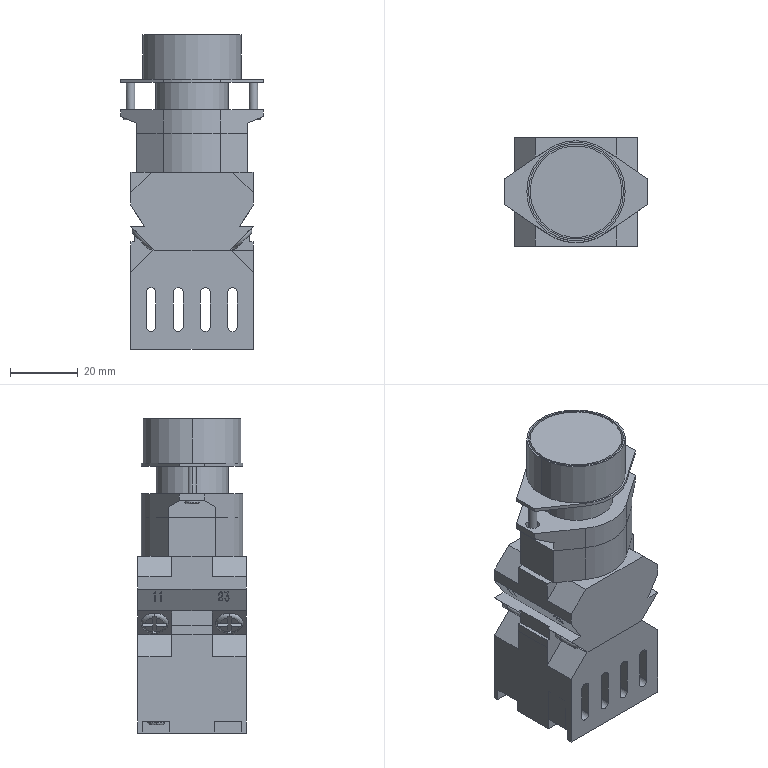Part | SolidWorks | features ICE 36, MirrorPattern 8, ConnectionPoint 4, Fillet 4, PLine 2, SmartComponentFeature 1 | 1 solid | 540 faces | box 42 x 32 x 92.5 mm | volume 74661 mm3 | plane 411 | spline 71 | cylinder 42 | torus 16 | commonest cylinder face diameters 2.937 x12 30 x6 2.5 x4 4 x4 4.3 x4 5 x4